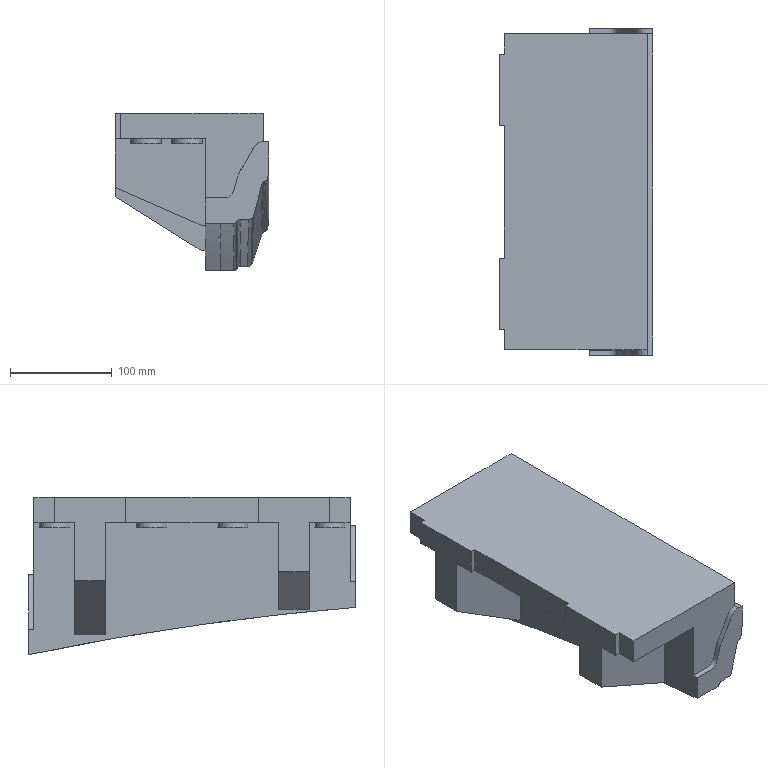Part | NX | features solid 2 | 1 solid | 56 faces | box 150.313 x 320 x 154.36 mm | volume 3360046 mm3 | plane 27 | spline 23 | cylinder 6 | commonest cylinder face diameters 30 x6